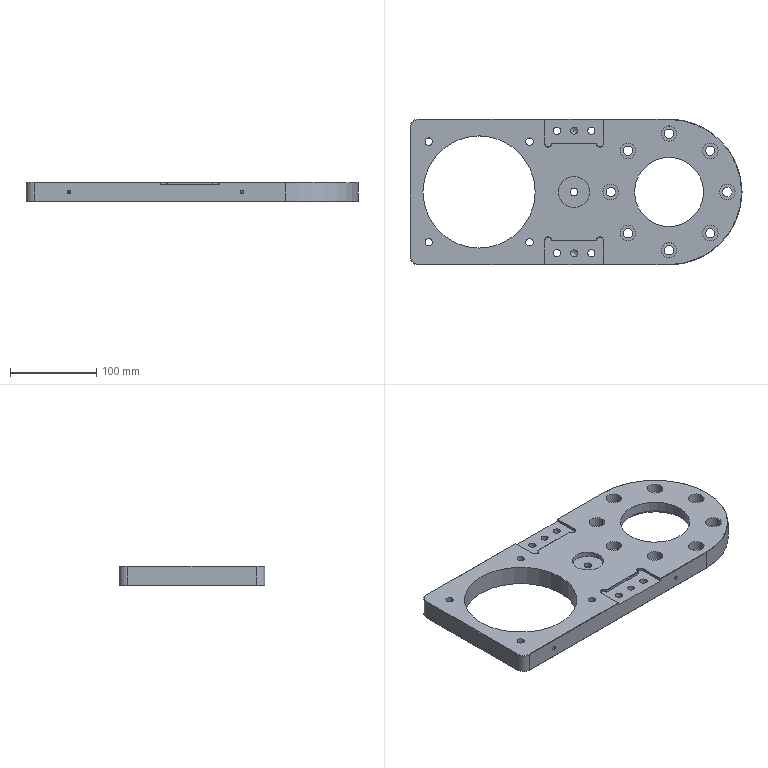Part | SolidWorks | features HoleWzd 7, ICE 7, MirrorPattern 5, Chamfer 2, CirPattern 1, Extrusion 1, Fillet 1 | 1 solid | 143 faces | box 384.5 x 169 x 23 mm | volume 899226 mm3 | cylinder 81 | plane 39 | cone 23 | commonest cylinder face diameters 8.5 x16 11 x16 18 x16 4.2 x8 8 x8 9 x2